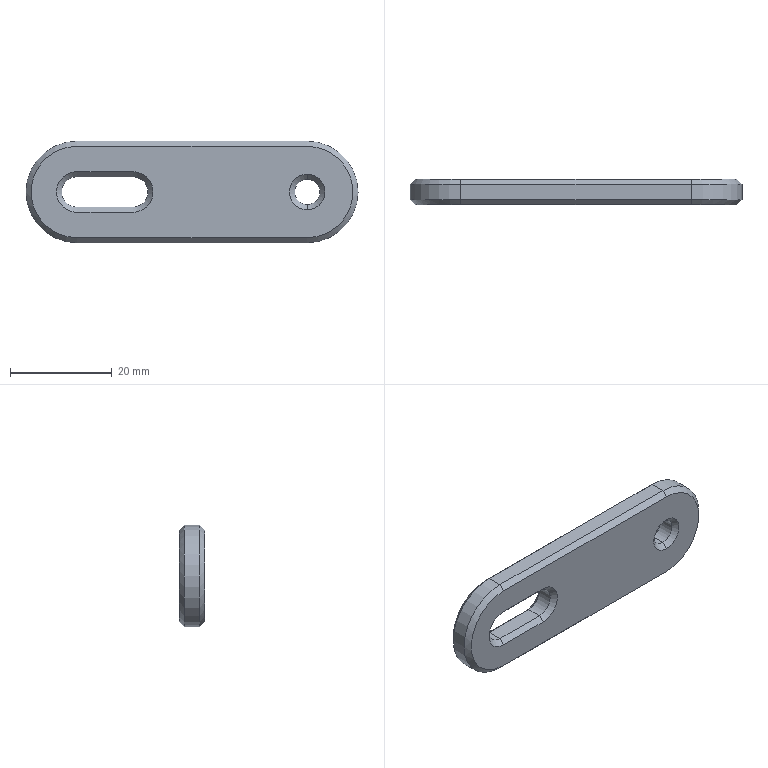Part | SolidWorks | features Chamfer 1, Extrusion 1 | 1 solid | 32 faces | box 65.398 x 5 x 20 mm | volume 5328 mm3 | plane 14 | cone 12 | cylinder 6 | commonest cylinder face diameters 5 x2 6 x2 20 x2
STEP:
#1=CARTESIAN_POINT('',(0.,4.,-2.5));
#2=VERTEX_POINT('',#1);
#3=CARTESIAN_POINT('',(0.,4.,2.5));
#4=VERTEX_POINT('',#3);
#5=CARTESIAN_POINT('',(0.,4.,0.));
#6=DIRECTION('',(0.,1.,0.));
#7=DIRECTION('',(0.,0.,1.));
#8=AXIS2_PLACEMENT_3D('',#5,#6,#7);
#9=CIRCLE('',#8,2.5);
#10=EDGE_CURVE('',#2,#4,#9,.T.);
#11=ORIENTED_EDGE('',*,*,#10,.F.);
#12=CARTESIAN_POINT('',(0.,5.,-3.5));
#13=VERTEX_POINT('',#12);
#14=CARTESIAN_POINT('',(0.,4.,-2.5));
#15=DIRECTION('',(0.,0.7071,-0.7071));
#16=VECTOR('',#15,1000.);
#17=LINE('',#14,#16);
#18=EDGE_CURVE('',#2,#13,#17,.T.);
#19=ORIENTED_EDGE('',*,*,#18,.T.);
#20=CARTESIAN_POINT('',(0.,5.,3.5));
#21=VERTEX_POINT('',#20);
#22=CARTESIAN_POINT('',(0.,5.,0.));
#23=DIRECTION('',(0.,-1.,0.));
#24=DIRECTION('',(0.,0.,1.));
#25=AXIS2_PLACEMENT_3D('',#22,#23,#24);
#26=CIRCLE('',#25,3.5);
#27=EDGE_CURVE('',#21,#13,#26,.T.);
#28=ORIENTED_EDGE('',*,*,#27,.F.);
#29=CARTESIAN_POINT('',(0.,4.,2.5));
#30=DIRECTION('',(0.,0.7071,0.7071));
#31=VECTOR('',#30,1000.);
#32=LINE('',#29,#31);
#33=EDGE_CURVE('',#4,#21,#32,.T.);
#34=ORIENTED_EDGE('',*,*,#33,.F.);
#35=EDGE_LOOP('',(#11,#19,#28,#34));
#36=FACE_OUTER_BOUND('',#35,.T.);
#37=CARTESIAN_POINT('',(0.,4.,0.));
#38=DIRECTION('',(0.,1.,0.));
#39=DIRECTION('',(0.,0.,1.));
#40=AXIS2_PLACEMENT_3D('',#37,#38,#39);
#41=CONICAL_SURFACE('',#40,2.5,0.7854);
#42=ADVANCED_FACE('',(#36),#41,.F.);
#43=CARTESIAN_POINT('',(0.,1.,2.5));
#44=VERTEX_POINT('',#43);
#45=CARTESIAN_POINT('',(0.,1.,-2.5));
#46=VERTEX_POINT('',#45);
#47=CARTESIAN_POINT('',(0.,1.,0.));
#48=DIRECTION('',(0.,-1.,0.));
#49=DIRECTION('',(0.,0.,1.));
#50=AXIS2_PLACEMENT_3D('',#47,#48,#49);
#51=CIRCLE('',#50,2.5);
#52=EDGE_CURVE('',#44,#46,#51,.T.);
#53=ORIENTED_EDGE('',*,*,#52,.F.);
#54=CARTESIAN_POINT('',(0.,0.,3.5));
#55=VERTEX_POINT('',#54);
#56=CARTESIAN_POINT('',(0.,0.,3.5));
#57=DIRECTION('',(0.,-0.7071,0.7071));
#58=VECTOR('',#57,1000.);
#59=LINE('',#56,#58);
#60=EDGE_CURVE('',#44,#55,#59,.T.);
#61=ORIENTED_EDGE('',*,*,#60,.T.);
#62=CARTESIAN_POINT('',(0.,0.,-3.5));
#63=VERTEX_POINT('',#62);
#64=CARTESIAN_POINT('',(0.,0.,0.));
#65=DIRECTION('',(0.,1.,0.));
#66=DIRECTION('',(0.,0.,1.));
#67=AXIS2_PLACEMENT_3D('',#64,#65,#66);
#68=CIRCLE('',#67,3.5);
#69=EDGE_CURVE('',#63,#55,#68,.T.);
#70=ORIENTED_EDGE('',*,*,#69,.F.);
#71=CARTESIAN_POINT('',(0.,0.,-3.5));
#72=DIRECTION('',(0.,-0.7071,-0.7071));
#73=VECTOR('',#72,1000.);
#74=LINE('',#71,#73);
#75=EDGE_CURVE('',#46,#63,#74,.T.);
#76=ORIENTED_EDGE('',*,*,#75,.F.);
#77=EDGE_LOOP('',(#53,#61,#70,#76));
#78=FACE_OUTER_BOUND('',#77,.T.);
#79=CARTESIAN_POINT('',(0.,0.,0.));
#80=DIRECTION('',(0.,-1.,0.));
#81=DIRECTION('',(0.,0.,-1.));
#82=AXIS2_PLACEMENT_3D('',#79,#80,#81);
#83=CONICAL_SURFACE('',#82,3.5,0.7854);
#84=ADVANCED_FACE('',(#78),#83,.F.);
#85=ORIENTED_EDGE('',*,*,#10,.T.);
#86=CARTESIAN_POINT('',(0.,5.,2.5));
#87=DIRECTION('',(0.,-1.,0.));
#88=VECTOR('',#87,1000.);
#89=LINE('',#86,#88);
#90=EDGE_CURVE('',#4,#44,#89,.T.);
#91=ORIENTED_EDGE('',*,*,#90,.T.);
#92=ORIENTED_EDGE('',*,*,#52,.T.);
#93=CARTESIAN_POINT('',(0.,5.,-2.5));
#94=DIRECTION('',(0.,-1.,0.));
#95=VECTOR('',#94,1000.);
#96=LINE('',#93,#95);
#97=EDGE_CURVE('',#2,#46,#96,.T.);
#98=ORIENTED_EDGE('',*,*,#97,.F.);
#99=EDGE_LOOP('',(#85,#91,#92,#98));
#100=FACE_OUTER_BOUND('',#99,.T.);
#101=CARTESIAN_POINT('',(0.,5.,0.));
#102=DIRECTION('',(0.,-1.,0.));
#103=DIRECTION('',(0.,0.,-1.));
#104=AXIS2_PLACEMENT_3D('',#101,#102,#103);
#105=CYLINDRICAL_SURFACE('',#104,2.5);
#106=ADVANCED_FACE('',(#100),#105,.F.);
#107=CARTESIAN_POINT('',(-45.398,5.,-4.));
#108=VERTEX_POINT('',#107);
#109=CARTESIAN_POINT('',(-34.373,5.,-4.));
#110=VERTEX_POINT('',#109);
#111=CARTESIAN_POINT('',(0.,5.,-4.));
#112=DIRECTION('',(1.,0.,0.));
#113=VECTOR('',#112,1000.);
#114=LINE('',#111,#113);
#115=EDGE_CURVE('',#108,#110,#114,.T.);
#116=ORIENTED_EDGE('',*,*,#115,.T.);
#117=CARTESIAN_POINT('',(-34.373,5.,4.));
#118=VERTEX_POINT('',#117);
#119=CARTESIAN_POINT('',(-34.373,5.,0.));
#120=DIRECTION('',(0.,-1.,0.));
#121=DIRECTION('',(0.,0.,1.));
#122=AXIS2_PLACEMENT_3D('',#119,#120,#121);
#123=CIRCLE('',#122,4.);
#124=EDGE_CURVE('',#110,#118,#123,.T.);
#125=ORIENTED_EDGE('',*,*,#124,.T.);
#126=CARTESIAN_POINT('',(-45.398,5.,4.));
#127=VERTEX_POINT('',#126);
#128=CARTESIAN_POINT('',(0.,5.,4.));
#129=DIRECTION('',(-1.,0.,0.));
#130=VECTOR('',#129,1000.);
#131=LINE('',#128,#130);
#132=EDGE_CURVE('',#118,#127,#131,.T.);
#133=ORIENTED_EDGE('',*,*,#132,.T.);
#134=CARTESIAN_POINT('',(-45.398,5.,0.));
#135=DIRECTION('',(0.,-1.,0.));
#136=DIRECTION('',(0.,0.,1.));
#137=AXIS2_PLACEMENT_3D('',#134,#135,#136);
#138=CIRCLE('',#137,4.);
#139=EDGE_CURVE('',#127,#108,#138,.T.);
#140=ORIENTED_EDGE('',*,*,#139,.T.);
#141=EDGE_LOOP('',(#116,#125,#133,#140));
#142=FACE_BOUND('',#141,.T.);
#143=ORIENTED_EDGE('',*,*,#27,.T.);
#144=CARTESIAN_POINT('',(0.,5.,0.));
#145=DIRECTION('',(0.,-1.,0.));
#146=DIRECTION('',(0.,0.,1.));
#147=AXIS2_PLACEMENT_3D('',#144,#145,#146);
#148=CIRCLE('',#147,3.5);
#149=EDGE_CURVE('',#13,#21,#148,.T.);
#150=ORIENTED_EDGE('',*,*,#149,.T.);
#151=EDGE_LOOP('',(#143,#150));
#152=FACE_BOUND('',#151,.T.);
#153=CARTESIAN_POINT('',(-45.398,5.,-9.));
#154=VERTEX_POINT('',#153);
#155=CARTESIAN_POINT('',(-45.398,5.,9.));
#156=VERTEX_POINT('',#155);
#157=CARTESIAN_POINT('',(-45.398,5.,0.));
#158=DIRECTION('',(0.,1.,0.));
#159=DIRECTION('',(0.,0.,1.));
#160=AXIS2_PLACEMENT_3D('',#157,#158,#159);
#161=CIRCLE('',#160,9.);
#162=EDGE_CURVE('',#154,#156,#161,.T.);
#163=ORIENTED_EDGE('',*,*,#162,.T.);
#164=CARTESIAN_POINT('',(0.,5.,9.));
#165=VERTEX_POINT('',#164);
#166=CARTESIAN_POINT('',(0.,5.,9.));
#167=DIRECTION('',(1.,0.,0.));
#168=VECTOR('',#167,1000.);
#169=LINE('',#166,#168);
#170=EDGE_CURVE('',#156,#165,#169,.T.);
#171=ORIENTED_EDGE('',*,*,#170,.T.);
#172=CARTESIAN_POINT('',(0.,5.,-9.));
#173=VERTEX_POINT('',#172);
#174=CARTESIAN_POINT('',(0.,5.,0.));
#175=DIRECTION('',(0.,1.,0.));
#176=DIRECTION('',(0.,0.,1.));
#177=AXIS2_PLACEMENT_3D('',#174,#175,#176);
#178=CIRCLE('',#177,9.);
#179=EDGE_CURVE('',#165,#173,#178,.T.);
#180=ORIENTED_EDGE('',*,*,#179,.T.);
#181=CARTESIAN_POINT('',(-45.398,5.,-9.));
#182=DIRECTION('',(-1.,0.,0.));
#183=VECTOR('',#182,1000.);
#184=LINE('',#181,#183);
#185=EDGE_CURVE('',#173,#154,#184,.T.);
#186=ORIENTED_EDGE('',*,*,#185,.T.);
#187=EDGE_LOOP('',(#163,#171,#180,#186));
#188=FACE_OUTER_BOUND('',#187,.T.);
#189=CARTESIAN_POINT('',(0.,5.,0.));
#190=DIRECTION('',(0.,1.,0.));
#191=DIRECTION('',(0.,0.,1.));
#192=AXIS2_PLACEMENT_3D('',#189,#190,#191);
#193=PLANE('',#192);
#194=ADVANCED_FACE('',(#142,#152,#188),#193,.T.);
#195=CARTESIAN_POINT('',(-34.373,0.,4.));
#196=VERTEX_POINT('',#195);
#197=CARTESIAN_POINT('',(-34.373,0.,-4.));
#198=VERTEX_POINT('',#197);
#199=CARTESIAN_POINT('',(-34.373,0.,0.));
#200=DIRECTION('',(0.,1.,0.));
#201=DIRECTION('',(0.,0.,1.));
#202=AXIS2_PLACEMENT_3D('',#199,#200,#201);
#203=CIRCLE('',#202,4.);
#204=EDGE_CURVE('',#196,#198,#203,.T.);
#205=ORIENTED_EDGE('',*,*,#204,.T.);
#206=CARTESIAN_POINT('',(-45.398,0.,-4.));
#207=VERTEX_POINT('',#206);
#208=CARTESIAN_POINT('',(-45.398,0.,-4.));
#209=DIRECTION('',(-1.,0.,0.));
#210=VECTOR('',#209,1000.);
#211=LINE('',#208,#210);
#212=EDGE_CURVE('',#198,#207,#211,.T.);
#213=ORIENTED_EDGE('',*,*,#212,.T.);
#214=CARTESIAN_POINT('',(-45.398,0.,4.));
#215=VERTEX_POINT('',#214);
#216=CARTESIAN_POINT('',(-45.398,0.,0.));
#217=DIRECTION('',(0.,1.,0.));
#218=DIRECTION('',(0.,0.,1.));
#219=AXIS2_PLACEMENT_3D('',#216,#217,#218);
#220=CIRCLE('',#219,4.);
#221=EDGE_CURVE('',#207,#215,#220,.T.);
#222=ORIENTED_EDGE('',*,*,#221,.T.);
#223=CARTESIAN_POINT('',(-34.373,0.,4.));
#224=DIRECTION('',(1.,0.,0.));
#225=VECTOR('',#224,1000.);
#226=LINE('',#223,#225);
#227=EDGE_CURVE('',#215,#196,#226,.T.);
#228=ORIENTED_EDGE('',*,*,#227,.T.);
#229=EDGE_LOOP('',(#205,#213,#222,#228));
#230=FACE_BOUND('',#229,.T.);
#231=CARTESIAN_POINT('',(-45.398,0.,9.));
#232=VERTEX_POINT('',#231);
#233=CARTESIAN_POINT('',(-45.398,0.,-9.));
#234=VERTEX_POINT('',#233);
#235=CARTESIAN_POINT('',(-45.398,0.,0.));
#236=DIRECTION('',(0.,-1.,0.));
#237=DIRECTION('',(0.,0.,1.));
#238=AXIS2_PLACEMENT_3D('',#235,#236,#237);
#239=CIRCLE('',#238,9.);
#240=EDGE_CURVE('',#232,#234,#239,.T.);
#241=ORIENTED_EDGE('',*,*,#240,.T.);
#242=CARTESIAN_POINT('',(0.,0.,-9.));
#243=VERTEX_POINT('',#242);
#244=CARTESIAN_POINT('',(0.,0.,-9.));
#245=DIRECTION('',(1.,0.,0.));
#246=VECTOR('',#245,1000.);
#247=LINE('',#244,#246);
#248=EDGE_CURVE('',#234,#243,#247,.T.);
#249=ORIENTED_EDGE('',*,*,#248,.T.);
#250=CARTESIAN_POINT('',(0.,0.,9.));
#251=VERTEX_POINT('',#250);
#252=CARTESIAN_POINT('',(0.,0.,0.));
#253=DIRECTION('',(0.,-1.,0.));
#254=DIRECTION('',(0.,0.,1.));
#255=AXIS2_PLACEMENT_3D('',#252,#253,#254);
#256=CIRCLE('',#255,9.);
#257=EDGE_CURVE('',#243,#251,#256,.T.);
#258=ORIENTED_EDGE('',*,*,#257,.T.);
#259=CARTESIAN_POINT('',(0.,0.,9.));
#260=DIRECTION('',(-1.,0.,0.));
#261=VECTOR('',#260,1000.);
#262=LINE('',#259,#261);
#263=EDGE_CURVE('',#251,#232,#262,.T.);
#264=ORIENTED_EDGE('',*,*,#263,.T.);
#265=EDGE_LOOP('',(#241,#249,#258,#264));
#266=FACE_OUTER_BOUND('',#265,.T.);
#267=ORIENTED_EDGE('',*,*,#69,.T.);
#268=CARTESIAN_POINT('',(0.,0.,0.));
#269=DIRECTION('',(0.,1.,0.));
#270=DIRECTION('',(0.,0.,1.));
#271=AXIS2_PLACEMENT_3D('',#268,#269,#270);
#272=CIRCLE('',#271,3.5);
#273=EDGE_CURVE('',#55,#63,#272,.T.);
#274=ORIENTED_EDGE('',*,*,#273,.T.);
#275=EDGE_LOOP('',(#267,#274));
#276=FACE_BOUND('',#275,.T.);
#277=CARTESIAN_POINT('',(0.,0.,0.));
#278=DIRECTION('',(0.,1.,0.));
#279=DIRECTION('',(0.,0.,1.));
#280=AXIS2_PLACEMENT_3D('',#277,#278,#279);
#281=PLANE('',#280);
#282=ADVANCED_FACE('',(#230,#266,#276),#281,.F.);
#283=CARTESIAN_POINT('',(0.,4.,10.));
#284=VERTEX_POINT('',#283);
#285=CARTESIAN_POINT('',(0.,1.,10.));
#286=VERTEX_POINT('',#285);
#287=CARTESIAN_POINT('',(0.,5.,10.));
#288=DIRECTION('',(0.,-1.,0.));
#289=VECTOR('',#288,1000.);
#290=LINE('',#287,#289);
#291=EDGE_CURVE('',#284,#286,#290,.T.);
#292=ORIENTED_EDGE('',*,*,#291,.T.);
#293=CARTESIAN_POINT('',(0.,1.,-10.));
#294=VERTEX_POINT('',#293);
#295=CARTESIAN_POINT('',(0.,1.,0.));
#296=DIRECTION('',(0.,1.,0.));
#297=DIRECTION('',(0.,0.,1.));
#298=AXIS2_PLACEMENT_3D('',#295,#296,#297);
#299=CIRCLE('',#298,10.);
#300=EDGE_CURVE('',#286,#294,#299,.T.);
#301=ORIENTED_EDGE('',*,*,#300,.T.);
#302=CARTESIAN_POINT('',(0.,4.,-10.));
#303=VERTEX_POINT('',#302);
#304=CARTESIAN_POINT('',(0.,5.,-10.));
#305=DIRECTION('',(0.,-1.,0.));
#306=VECTOR('',#305,1000.);
#307=LINE('',#304,#306);
#308=EDGE_CURVE('',#303,#294,#307,.T.);
#309=ORIENTED_EDGE('',*,*,#308,.F.);
#310=CARTESIAN_POINT('',(0.,4.,0.));
#311=DIRECTION('',(0.,-1.,0.));
#312=DIRECTION('',(0.,0.,1.));
#313=AXIS2_PLACEMENT_3D('',#310,#311,#312);
#314=CIRCLE('',#313,10.);
#315=EDGE_CURVE('',#303,#284,#314,.T.);
#316=ORIENTED_EDGE('',*,*,#315,.T.);
#317=EDGE_LOOP('',(#292,#301,#309,#316));
#318=FACE_OUTER_BOUND('',#317,.T.);
#319=CARTESIAN_POINT('',(0.,5.,0.));
#320=DIRECTION('',(0.,-1.,0.));
#321=DIRECTION('',(0.,0.,-1.));
#322=AXIS2_PLACEMENT_3D('',#319,#320,#321);
#323=CYLINDRICAL_SURFACE('',#322,10.);
#324=ADVANCED_FACE('',(#318),#323,.T.);
#325=ORIENTED_EDGE('',*,*,#308,.T.);
#326=CARTESIAN_POINT('',(-45.398,1.,-10.));
#327=VERTEX_POINT('',#326);
#328=CARTESIAN_POINT('',(0.,1.,-10.));
#329=DIRECTION('',(-1.,0.,0.));
#330=VECTOR('',#329,1000.);
#331=LINE('',#328,#330);
#332=EDGE_CURVE('',#294,#327,#331,.T.);
#333=ORIENTED_EDGE('',*,*,#332,.T.);
#334=CARTESIAN_POINT('',(-45.398,4.,-10.));
#335=VERTEX_POINT('',#334);
#336=CARTESIAN_POINT('',(-45.398,5.,-10.));
#337=DIRECTION('',(0.,-1.,0.));
#338=VECTOR('',#337,1000.);
#339=LINE('',#336,#338);
#340=EDGE_CURVE('',#335,#327,#339,.T.);
#341=ORIENTED_EDGE('',*,*,#340,.F.);
#342=CARTESIAN_POINT('',(0.,4.,-10.));
#343=DIRECTION('',(1.,0.,0.));
#344=VECTOR('',#343,1000.);
#345=LINE('',#342,#344);
#346=EDGE_CURVE('',#335,#303,#345,.T.);
#347=ORIENTED_EDGE('',*,*,#346,.T.);
#348=EDGE_LOOP('',(#325,#333,#341,#347));
#349=FACE_OUTER_BOUND('',#348,.T.);
#350=CARTESIAN_POINT('',(0.,5.,-10.));
#351=DIRECTION('',(0.,0.,1.));
#352=DIRECTION('',(1.,0.,0.));
#353=AXIS2_PLACEMENT_3D('',#350,#351,#352);
#354=PLANE('',#353);
#355=ADVANCED_FACE('',(#349),#354,.F.);
#356=ORIENTED_EDGE('',*,*,#340,.T.);
#357=CARTESIAN_POINT('',(-45.398,1.,10.));
#358=VERTEX_POINT('',#357);
#359=CARTESIAN_POINT('',(-45.398,1.,0.));
#360=DIRECTION('',(0.,1.,0.));
#361=DIRECTION('',(0.,0.,1.));
#362=AXIS2_PLACEMENT_3D('',#359,#360,#361);
#363=CIRCLE('',#362,10.);
#364=EDGE_CURVE('',#327,#358,#363,.T.);
#365=ORIENTED_EDGE('',*,*,#364,.T.);
#366=CARTESIAN_POINT('',(-45.398,4.,10.));
#367=VERTEX_POINT('',#366);
#368=CARTESIAN_POINT('',(-45.398,5.,10.));
#369=DIRECTION('',(0.,-1.,0.));
#370=VECTOR('',#369,1000.);
#371=LINE('',#368,#370);
#372=EDGE_CURVE('',#367,#358,#371,.T.);
#373=ORIENTED_EDGE('',*,*,#372,.F.);
#374=CARTESIAN_POINT('',(-45.398,4.,0.));
#375=DIRECTION('',(0.,-1.,0.));
#376=DIRECTION('',(0.,0.,1.));
#377=AXIS2_PLACEMENT_3D('',#374,#375,#376);
#378=CIRCLE('',#377,10.);
#379=EDGE_CURVE('',#367,#335,#378,.T.);
#380=ORIENTED_EDGE('',*,*,#379,.T.);
#381=EDGE_LOOP('',(#356,#365,#373,#380));
#382=FACE_OUTER_BOUND('',#381,.T.);
#383=CARTESIAN_POINT('',(-45.398,5.,0.));
#384=DIRECTION('',(0.,-1.,0.));
#385=DIRECTION('',(0.,0.,-1.));
#386=AXIS2_PLACEMENT_3D('',#383,#384,#385);
#387=CYLINDRICAL_SURFACE('',#386,10.);
#388=ADVANCED_FACE('',(#382),#387,.T.);
#389=ORIENTED_EDGE('',*,*,#372,.T.);
#390=CARTESIAN_POINT('',(0.,1.,10.));
#391=DIRECTION('',(1.,0.,0.));
#392=VECTOR('',#391,1000.);
#393=LINE('',#390,#392);
#394=EDGE_CURVE('',#358,#286,#393,.T.);
#395=ORIENTED_EDGE('',*,*,#394,.T.);
#396=ORIENTED_EDGE('',*,*,#291,.F.);
#397=CARTESIAN_POINT('',(-45.398,4.,10.));
#398=DIRECTION('',(-1.,0.,0.));
#399=VECTOR('',#398,1000.);
#400=LINE('',#397,#399);
#401=EDGE_CURVE('',#284,#367,#400,.T.);
#402=ORIENTED_EDGE('',*,*,#401,.T.);
#403=EDGE_LOOP('',(#389,#395,#396,#402));
#404=FACE_OUTER_BOUND('',#403,.T.);
#405=CARTESIAN_POINT('',(0.,5.,10.));
#406=DIRECTION('',(0.,0.,-1.));
#407=DIRECTION('',(-1.,0.,0.));
#408=AXIS2_PLACEMENT_3D('',#405,#406,#407);
#409=PLANE('',#408);
#410=ADVANCED_FACE('',(#404),#409,.F.);
#411=ORIENTED_EDGE('',*,*,#90,.F.);
#412=CARTESIAN_POINT('',(0.,4.,0.));
#413=DIRECTION('',(0.,1.,0.));
#414=DIRECTION('',(0.,0.,1.));
#415=AXIS2_PLACEMENT_3D('',#412,#413,#414);
#416=CIRCLE('',#415,2.5);
#417=EDGE_CURVE('',#4,#2,#416,.T.);
#418=ORIENTED_EDGE('',*,*,#417,.T.);
#419=ORIENTED_EDGE('',*,*,#97,.T.);
#420=CARTESIAN_POINT('',(0.,1.,0.));
#421=DIRECTION('',(0.,-1.,0.));
#422=DIRECTION('',(0.,0.,1.));
#423=AXIS2_PLACEMENT_3D('',#420,#421,#422);
#424=CIRCLE('',#423,2.5);
#425=EDGE_CURVE('',#46,#44,#424,.T.);
#426=ORIENTED_EDGE('',*,*,#425,.T.);
#427=EDGE_LOOP('',(#411,#418,#419,#426));
#428=FACE_OUTER_BOUND('',#427,.T.);
#429=CARTESIAN_POINT('',(0.,5.,0.));
#430=DIRECTION('',(0.,-1.,0.));
#431=DIRECTION('',(0.,0.,-1.));
#432=AXIS2_PLACEMENT_3D('',#429,#430,#431);
#433=CYLINDRICAL_SURFACE('',#432,2.5);
#434=ADVANCED_FACE('',(#428),#433,.F.);
#435=CARTESIAN_POINT('',(-45.398,4.,3.));
#436=VERTEX_POINT('',#435);
#437=CARTESIAN_POINT('',(-45.398,1.,3.));
#438=VERTEX_POINT('',#437);
#439=CARTESIAN_POINT('',(-45.398,5.,3.));
#440=DIRECTION('',(0.,-1.,0.));
#441=VECTOR('',#440,1000.);
#442=LINE('',#439,#441);
#443=EDGE_CURVE('',#436,#438,#442,.T.);
#444=ORIENTED_EDGE('',*,*,#443,.T.);
#445=CARTESIAN_POINT('',(-45.398,1.,-3.));
#446=VERTEX_POINT('',#445);
#447=CARTESIAN_POINT('',(-45.398,1.,0.));
#448=DIRECTION('',(0.,-1.,0.));
#449=DIRECTION('',(0.,0.,1.));
#450=AXIS2_PLACEMENT_3D('',#447,#448,#449);
#451=CIRCLE('',#450,3.);
#452=EDGE_CURVE('',#438,#446,#451,.T.);
#453=ORIENTED_EDGE('',*,*,#452,.T.);
#454=CARTESIAN_POINT('',(-45.398,4.,-3.));
#455=VERTEX_POINT('',#454);
#456=CARTESIAN_POINT('',(-45.398,5.,-3.));
#457=DIRECTION('',(0.,-1.,0.));
#458=VECTOR('',#457,1000.);
#459=LINE('',#456,#458);
#460=EDGE_CURVE('',#455,#446,#459,.T.);
#461=ORIENTED_EDGE('',*,*,#460,.F.);
#462=CARTESIAN_POINT('',(-45.398,4.,0.));
#463=DIRECTION('',(0.,1.,0.));
#464=DIRECTION('',(0.,0.,1.));
#465=AXIS2_PLACEMENT_3D('',#462,#463,#464);
#466=CIRCLE('',#465,3.);
#467=EDGE_CURVE('',#455,#436,#466,.T.);
#468=ORIENTED_EDGE('',*,*,#467,.T.);
#469=EDGE_LOOP('',(#444,#453,#461,#468));
#470=FACE_OUTER_BOUND('',#469,.T.);
#471=CARTESIAN_POINT('',(-45.398,5.,0.));
#472=DIRECTION('',(0.,-1.,0.));
#473=DIRECTION('',(0.,0.,-1.));
#474=AXIS2_PLACEMENT_3D('',#471,#472,#473);
#475=CYLINDRICAL_SURFACE('',#474,3.);
#476=ADVANCED_FACE('',(#470),#475,.F.);
#477=CARTESIAN_POINT('',(-34.373,4.,3.));
#478=VERTEX_POINT('',#477);
#479=CARTESIAN_POINT('',(-34.373,1.,3.));
#480=VERTEX_POINT('',#479);
#481=CARTESIAN_POINT('',(-34.373,5.,3.));
#482=DIRECTION('',(0.,-1.,0.));
#483=VECTOR('',#482,1000.);
#484=LINE('',#481,#483);
#485=EDGE_CURVE('',#478,#480,#484,.T.);
#486=ORIENTED_EDGE('',*,*,#485,.T.);
#487=CARTESIAN_POINT('',(-45.398,1.,3.));
#488=DIRECTION('',(-1.,0.,0.));
#489=VECTOR('',#488,1000.);
#490=LINE('',#487,#489);
#491=EDGE_CURVE('',#480,#438,#490,.T.);
#492=ORIENTED_EDGE('',*,*,#491,.T.);
#493=ORIENTED_EDGE('',*,*,#443,.F.);
#494=CARTESIAN_POINT('',(-45.398,4.,3.));
#495=DIRECTION('',(1.,0.,0.));
#496=VECTOR('',#495,1000.);
#497=LINE('',#494,#496);
#498=EDGE_CURVE('',#436,#478,#497,.T.);
#499=ORIENTED_EDGE('',*,*,#498,.T.);
#500=EDGE_LOOP('',(#486,#492,#493,#499));
#501=FACE_OUTER_BOUND('',#500,.T.);
#502=CARTESIAN_POINT('',(-45.398,5.,3.));
#503=DIRECTION('',(0.,0.,-1.));
#504=DIRECTION('',(-1.,0.,0.));
#505=AXIS2_PLACEMENT_3D('',#502,#503,#504);
#506=PLANE('',#505);
#507=ADVANCED_FACE('',(#501),#506,.T.);
#508=CARTESIAN_POINT('',(-34.373,4.,-3.));
#509=VERTEX_POINT('',#508);
#510=CARTESIAN_POINT('',(-34.373,1.,-3.));
#511=VERTEX_POINT('',#510);
#512=CARTESIAN_POINT('',(-34.373,5.,-3.));
#513=DIRECTION('',(0.,-1.,0.));
#514=VECTOR('',#513,1000.);
#515=LINE('',#512,#514);
#516=EDGE_CURVE('',#509,#511,#515,.T.);
#517=ORIENTED_EDGE('',*,*,#516,.T.);
#518=CARTESIAN_POINT('',(-34.373,1.,0.));
#519=DIRECTION('',(0.,-1.,0.));
#520=DIRECTION('',(0.,0.,1.));
#521=AXIS2_PLACEMENT_3D('',#518,#519,#520);
#522=CIRCLE('',#521,3.);
#523=EDGE_CURVE('',#511,#480,#522,.T.);
#524=ORIENTED_EDGE('',*,*,#523,.T.);
#525=ORIENTED_EDGE('',*,*,#485,.F.);
#526=CARTESIAN_POINT('',(-34.373,4.,0.));
#527=DIRECTION('',(0.,1.,0.));
#528=DIRECTION('',(0.,0.,1.));
#529=AXIS2_PLACEMENT_3D('',#526,#527,#528);
#530=CIRCLE('',#529,3.);
#531=EDGE_CURVE('',#478,#509,#530,.T.);
#532=ORIENTED_EDGE('',*,*,#531,.T.);
#533=EDGE_LOOP('',(#517,#524,#525,#532));
#534=FACE_OUTER_BOUND('',#533,.T.);
#535=CARTESIAN_POINT('',(-34.373,5.,0.));
#536=DIRECTION('',(0.,-1.,0.));
#537=DIRECTION('',(0.,0.,-1.));
#538=AXIS2_PLACEMENT_3D('',#535,#536,#537);
#539=CYLINDRICAL_SURFACE('',#538,3.);
#540=ADVANCED_FACE('',(#534),#539,.F.);
#541=ORIENTED_EDGE('',*,*,#460,.T.);
#542=CARTESIAN_POINT('',(-34.373,1.,-3.));
#543=DIRECTION('',(1.,0.,0.));
#544=VECTOR('',#543,1000.);
#545=LINE('',#542,#544);
#546=EDGE_CURVE('',#446,#511,#545,.T.);
#547=ORIENTED_EDGE('',*,*,#546,.T.);
#548=ORIENTED_EDGE('',*,*,#516,.F.);
#549=CARTESIAN_POINT('',(-45.398,4.,-3.));
#550=DIRECTION('',(-1.,0.,0.));
#551=VECTOR('',#550,1000.);
#552=LINE('',#549,#551);
#553=EDGE_CURVE('',#509,#455,#552,.T.);
#554=ORIENTED_EDGE('',*,*,#553,.T.);
#555=EDGE_LOOP('',(#541,#547,#548,#554));
#556=FACE_OUTER_BOUND('',#555,.T.);
#557=CARTESIAN_POINT('',(-45.398,5.,-3.));
#558=DIRECTION('',(0.,0.,1.));
#559=DIRECTION('',(1.,0.,0.));
#560=AXIS2_PLACEMENT_3D('',#557,#558,#559);
#561=PLANE('',#560);
#562=ADVANCED_FACE('',(#556),#561,.T.);
#563=CARTESIAN_POINT('',(-45.398,1.,3.));
#564=DIRECTION('',(0.,-0.7071,0.7071));
#565=VECTOR('',#564,1000.);
#566=LINE('',#563,#565);
#567=EDGE_CURVE('',#438,#215,#566,.T.);
#568=ORIENTED_EDGE('',*,*,#567,.F.);
#569=ORIENTED_EDGE('',*,*,#491,.F.);
#570=CARTESIAN_POINT('',(-34.373,0.,4.));
#571=DIRECTION('',(0.,0.7071,-0.7071));
#572=VECTOR('',#571,1000.);
#573=LINE('',#570,#572);
#574=EDGE_CURVE('',#196,#480,#573,.T.);
#575=ORIENTED_EDGE('',*,*,#574,.F.);
#576=ORIENTED_EDGE('',*,*,#227,.F.);
#577=EDGE_LOOP('',(#568,#569,#575,#576));
#578=FACE_OUTER_BOUND('',#577,.T.);
#579=CARTESIAN_POINT('',(0.,0.,4.));
#580=DIRECTION('',(0.,-0.7071,-0.7071));
#581=DIRECTION('',(-1.,0.,0.));
#582=AXIS2_PLACEMENT_3D('',#579,#580,#581);
#583=PLANE('',#582);
#584=ADVANCED_FACE('',(#578),#583,.T.);
#585=ORIENTED_EDGE('',*,*,#574,.T.);
#586=ORIENTED_EDGE('',*,*,#523,.F.);
#587=CARTESIAN_POINT('',(-34.373,0.,-4.));
#588=DIRECTION('',(0.,0.7071,0.7071));
#589=VECTOR('',#588,1000.);
#590=LINE('',#587,#589);
#591=EDGE_CURVE('',#198,#511,#590,.T.);
#592=ORIENTED_EDGE('',*,*,#591,.F.);
#593=ORIENTED_EDGE('',*,*,#204,.F.);
#594=EDGE_LOOP('',(#585,#586,#592,#593));
#595=FACE_OUTER_BOUND('',#594,.T.);
#596=CARTESIAN_POINT('',(-34.373,0.,0.));
#597=DIRECTION('',(0.,-1.,0.));
#598=DIRECTION('',(0.,0.,-1.));
#599=AXIS2_PLACEMENT_3D('',#596,#597,#598);
#600=CONICAL_SURFACE('',#599,4.,0.7854);
#601=ADVANCED_FACE('',(#595),#600,.F.);
#602=ORIENTED_EDGE('',*,*,#567,.T.);
#603=ORIENTED_EDGE('',*,*,#221,.F.);
#604=CARTESIAN_POINT('',(-45.398,1.,-3.));
#605=DIRECTION('',(0.,-0.7071,-0.7071));
#606=VECTOR('',#605,1000.);
#607=LINE('',#604,#606);
#608=EDGE_CURVE('',#446,#207,#607,.T.);
#609=ORIENTED_EDGE('',*,*,#608,.F.);
#610=ORIENTED_EDGE('',*,*,#452,.F.);
#611=EDGE_LOOP('',(#602,#603,#609,#610));
#612=FACE_OUTER_BOUND('',#611,.T.);
#613=CARTESIAN_POINT('',(-45.398,0.,0.));
#614=DIRECTION('',(0.,-1.,0.));
#615=DIRECTION('',(0.,0.,-1.));
#616=AXIS2_PLACEMENT_3D('',#613,#614,#615);
#617=CONICAL_SURFACE('',#616,4.,0.7854);
#618=ADVANCED_FACE('',(#612),#617,.F.);
#619=ORIENTED_EDGE('',*,*,#591,.T.);
#620=ORIENTED_EDGE('',*,*,#546,.F.);
#621=ORIENTED_EDGE('',*,*,#608,.T.);
#622=ORIENTED_EDGE('',*,*,#212,.F.);
#623=EDGE_LOOP('',(#619,#620,#621,#622));
#624=FACE_OUTER_BOUND('',#623,.T.);
#625=CARTESIAN_POINT('',(0.,0.,-4.));
#626=DIRECTION('',(0.,-0.7071,0.7071));
#627=DIRECTION('',(1.,0.,0.));
#628=AXIS2_PLACEMENT_3D('',#625,#626,#627);
#629=PLANE('',#628);
#630=ADVANCED_FACE('',(#624),#629,.T.);
#631=CARTESIAN_POINT('',(-45.398,0.,9.));
#632=DIRECTION('',(0.,0.7071,0.7071));
#633=VECTOR('',#632,1000.);
#634=LINE('',#631,#633);
#635=EDGE_CURVE('',#232,#358,#634,.T.);
#636=ORIENTED_EDGE('',*,*,#635,.F.);
#637=ORIENTED_EDGE('',*,*,#263,.F.);
#638=CARTESIAN_POINT('',(0.,1.,10.));
#639=DIRECTION('',(0.,-0.7071,-0.7071));
#640=VECTOR('',#639,1000.);
#641=LINE('',#638,#640);
#642=EDGE_CURVE('',#286,#251,#641,.T.);
#643=ORIENTED_EDGE('',*,*,#642,.F.);
#644=ORIENTED_EDGE('',*,*,#394,.F.);
#645=EDGE_LOOP('',(#636,#637,#643,#644));
#646=FACE_OUTER_BOUND('',#645,.T.);
#647=CARTESIAN_POINT('',(0.,1.,10.));
#648=DIRECTION('',(0.,0.7071,-0.7071));
#649=DIRECTION('',(1.,0.,0.));
#650=AXIS2_PLACEMENT_3D('',#647,#648,#649);
#651=PLANE('',#650);
#652=ADVANCED_FACE('',(#646),#651,.F.);
#653=ORIENTED_EDGE('',*,*,#642,.T.);
#654=ORIENTED_EDGE('',*,*,#257,.F.);
#655=CARTESIAN_POINT('',(0.,1.,-10.));
#656=DIRECTION('',(0.,-0.7071,0.7071));
#657=VECTOR('',#656,1000.);
#658=LINE('',#655,#657);
#659=EDGE_CURVE('',#294,#243,#658,.T.);
#660=ORIENTED_EDGE('',*,*,#659,.F.);
#661=ORIENTED_EDGE('',*,*,#300,.F.);
#662=EDGE_LOOP('',(#653,#654,#660,#661));
#663=FACE_OUTER_BOUND('',#662,.T.);
#664=CARTESIAN_POINT('',(0.,1.,0.));
#665=DIRECTION('',(0.,1.,0.));
#666=DIRECTION('',(0.,0.,1.));
#667=AXIS2_PLACEMENT_3D('',#664,#665,#666);
#668=CONICAL_SURFACE('',#667,10.,0.7854);
#669=ADVANCED_FACE('',(#663),#668,.T.);
#670=ORIENTED_EDGE('',*,*,#635,.T.);
#671=ORIENTED_EDGE('',*,*,#364,.F.);
#672=CARTESIAN_POINT('',(-45.398,0.,-9.));
#673=DIRECTION('',(0.,0.7071,-0.7071));
#674=VECTOR('',#673,1000.);
#675=LINE('',#672,#674);
#676=EDGE_CURVE('',#234,#327,#675,.T.);
#677=ORIENTED_EDGE('',*,*,#676,.F.);
#678=ORIENTED_EDGE('',*,*,#240,.F.);
#679=EDGE_LOOP('',(#670,#671,#677,#678));
#680=FACE_OUTER_BOUND('',#679,.T.);
#681=CARTESIAN_POINT('',(-45.398,1.,0.));
#682=DIRECTION('',(0.,1.,0.));
#683=DIRECTION('',(0.,0.,1.));
#684=AXIS2_PLACEMENT_3D('',#681,#682,#683);
#685=CONICAL_SURFACE('',#684,10.,0.7854);
#686=ADVANCED_FACE('',(#680),#685,.T.);
#687=ORIENTED_EDGE('',*,*,#659,.T.);
#688=ORIENTED_EDGE('',*,*,#248,.F.);
#689=ORIENTED_EDGE('',*,*,#676,.T.);
#690=ORIENTED_EDGE('',*,*,#332,.F.);
#691=EDGE_LOOP('',(#687,#688,#689,#690));
#692=FACE_OUTER_BOUND('',#691,.T.);
#693=CARTESIAN_POINT('',(0.,1.,-10.));
#694=DIRECTION('',(0.,0.7071,0.7071));
#695=DIRECTION('',(-1.,0.,0.));
#696=AXIS2_PLACEMENT_3D('',#693,#694,#695);
#697=PLANE('',#696);
#698=ADVANCED_FACE('',(#692),#697,.F.);
#699=ORIENTED_EDGE('',*,*,#60,.F.);
#700=ORIENTED_EDGE('',*,*,#425,.F.);
#701=ORIENTED_EDGE('',*,*,#75,.T.);
#702=ORIENTED_EDGE('',*,*,#273,.F.);
#703=EDGE_LOOP('',(#699,#700,#701,#702));
#704=FACE_OUTER_BOUND('',#703,.T.);
#705=CARTESIAN_POINT('',(0.,0.,0.));
#706=DIRECTION('',(0.,-1.,0.));
#707=DIRECTION('',(0.,0.,-1.));
#708=AXIS2_PLACEMENT_3D('',#705,#706,#707);
#709=CONICAL_SURFACE('',#708,3.5,0.7854);
#710=ADVANCED_FACE('',(#704),#709,.F.);
#711=CARTESIAN_POINT('',(-45.398,5.,-4.));
#712=DIRECTION('',(0.,-0.7071,0.7071));
#713=VECTOR('',#712,1000.);
#714=LINE('',#711,#713);
#715=EDGE_CURVE('',#108,#455,#714,.T.);
#716=ORIENTED_EDGE('',*,*,#715,.F.);
#717=ORIENTED_EDGE('',*,*,#139,.F.);
#718=CARTESIAN_POINT('',(-45.398,4.,3.));
#719=DIRECTION('',(0.,0.7071,0.7071));
#720=VECTOR('',#719,1000.);
#721=LINE('',#718,#720);
#722=EDGE_CURVE('',#436,#127,#721,.T.);
#723=ORIENTED_EDGE('',*,*,#722,.F.);
#724=ORIENTED_EDGE('',*,*,#467,.F.);
#725=EDGE_LOOP('',(#716,#717,#723,#724));
#726=FACE_OUTER_BOUND('',#725,.T.);
#727=CARTESIAN_POINT('',(-45.398,4.,0.));
#728=DIRECTION('',(0.,1.,0.));
#729=DIRECTION('',(0.,0.,1.));
#730=AXIS2_PLACEMENT_3D('',#727,#728,#729);
#731=CONICAL_SURFACE('',#730,3.,0.7854);
#732=ADVANCED_FACE('',(#726),#731,.F.);
#733=ORIENTED_EDGE('',*,*,#722,.T.);
#734=ORIENTED_EDGE('',*,*,#132,.F.);
#735=CARTESIAN_POINT('',(-34.373,4.,3.));
#736=DIRECTION('',(0.,0.7071,0.7071));
#737=VECTOR('',#736,1000.);
#738=LINE('',#735,#737);
#739=EDGE_CURVE('',#478,#118,#738,.T.);
#740=ORIENTED_EDGE('',*,*,#739,.F.);
#741=ORIENTED_EDGE('',*,*,#498,.F.);
#742=EDGE_LOOP('',(#733,#734,#740,#741));
#743=FACE_OUTER_BOUND('',#742,.T.);
#744=CARTESIAN_POINT('',(-45.398,4.,3.));
#745=DIRECTION('',(0.,-0.7071,0.7071));
#746=DIRECTION('',(1.,0.,0.));
#747=AXIS2_PLACEMENT_3D('',#744,#745,#746);
#748=PLANE('',#747);
#749=ADVANCED_FACE('',(#743),#748,.F.);
#750=ORIENTED_EDGE('',*,*,#715,.T.);
#751=ORIENTED_EDGE('',*,*,#553,.F.);
#752=CARTESIAN_POINT('',(-34.373,5.,-4.));
#753=DIRECTION('',(0.,-0.7071,0.7071));
#754=VECTOR('',#753,1000.);
#755=LINE('',#752,#754);
#756=EDGE_CURVE('',#110,#509,#755,.T.);
#757=ORIENTED_EDGE('',*,*,#756,.F.);
#758=ORIENTED_EDGE('',*,*,#115,.F.);
#759=EDGE_LOOP('',(#750,#751,#757,#758));
#760=FACE_OUTER_BOUND('',#759,.T.);
#761=CARTESIAN_POINT('',(-45.398,4.,-3.));
#762=DIRECTION('',(0.,-0.7071,-0.7071));
#763=DIRECTION('',(-1.,0.,0.));
#764=AXIS2_PLACEMENT_3D('',#761,#762,#763);
#765=PLANE('',#764);
#766=ADVANCED_FACE('',(#760),#765,.F.);
#767=ORIENTED_EDGE('',*,*,#739,.T.);
#768=ORIENTED_EDGE('',*,*,#124,.F.);
#769=ORIENTED_EDGE('',*,*,#756,.T.);
#770=ORIENTED_EDGE('',*,*,#531,.F.);
#771=EDGE_LOOP('',(#767,#768,#769,#770));
#772=FACE_OUTER_BOUND('',#771,.T.);
#773=CARTESIAN_POINT('',(-34.373,4.,0.));
#774=DIRECTION('',(0.,1.,0.));
#775=DIRECTION('',(0.,0.,1.));
#776=AXIS2_PLACEMENT_3D('',#773,#774,#775);
#777=CONICAL_SURFACE('',#776,3.,0.7854);
#778=ADVANCED_FACE('',(#772),#777,.F.);
#779=ORIENTED_EDGE('',*,*,#18,.F.);
#780=ORIENTED_EDGE('',*,*,#417,.F.);
#781=ORIENTED_EDGE('',*,*,#33,.T.);
#782=ORIENTED_EDGE('',*,*,#149,.F.);
#783=EDGE_LOOP('',(#779,#780,#781,#782));
#784=FACE_OUTER_BOUND('',#783,.T.);
#785=CARTESIAN_POINT('',(0.,4.,0.));
#786=DIRECTION('',(0.,1.,0.));
#787=DIRECTION('',(0.,0.,1.));
#788=AXIS2_PLACEMENT_3D('',#785,#786,#787);
#789=CONICAL_SURFACE('',#788,2.5,0.7854);
#790=ADVANCED_FACE('',(#784),#789,.F.);
#791=CARTESIAN_POINT('',(0.,4.,-10.));
#792=DIRECTION('',(0.,0.7071,0.7071));
#793=VECTOR('',#792,1000.);
#794=LINE('',#791,#793);
#795=EDGE_CURVE('',#303,#173,#794,.T.);
#796=ORIENTED_EDGE('',*,*,#795,.F.);
#797=ORIENTED_EDGE('',*,*,#346,.F.);
#798=CARTESIAN_POINT('',(-45.398,5.,-9.));
#799=DIRECTION('',(0.,-0.7071,-0.7071));
#800=VECTOR('',#799,1000.);
#801=LINE('',#798,#800);
#802=EDGE_CURVE('',#154,#335,#801,.T.);
#803=ORIENTED_EDGE('',*,*,#802,.F.);
#804=ORIENTED_EDGE('',*,*,#185,.F.);
#805=EDGE_LOOP('',(#796,#797,#803,#804));
#806=FACE_OUTER_BOUND('',#805,.T.);
#807=CARTESIAN_POINT('',(0.,5.,-9.));
#808=DIRECTION('',(0.,0.7071,-0.7071));
#809=DIRECTION('',(1.,0.,0.));
#810=AXIS2_PLACEMENT_3D('',#807,#808,#809);
#811=PLANE('',#810);
#812=ADVANCED_FACE('',(#806),#811,.T.);
#813=ORIENTED_EDGE('',*,*,#802,.T.);
#814=ORIENTED_EDGE('',*,*,#379,.F.);
#815=CARTESIAN_POINT('',(-45.398,5.,9.));
#816=DIRECTION('',(0.,-0.7071,0.7071));
#817=VECTOR('',#816,1000.);
#818=LINE('',#815,#817);
#819=EDGE_CURVE('',#156,#367,#818,.T.);
#820=ORIENTED_EDGE('',*,*,#819,.F.);
#821=ORIENTED_EDGE('',*,*,#162,.F.);
#822=EDGE_LOOP('',(#813,#814,#820,#821));
#823=FACE_OUTER_BOUND('',#822,.T.);
#824=CARTESIAN_POINT('',(-45.398,5.,0.));
#825=DIRECTION('',(0.,-1.,0.));
#826=DIRECTION('',(0.,0.,-1.));
#827=AXIS2_PLACEMENT_3D('',#824,#825,#826);
#828=CONICAL_SURFACE('',#827,9.,0.7854);
#829=ADVANCED_FACE('',(#823),#828,.T.);
#830=ORIENTED_EDGE('',*,*,#795,.T.);
#831=ORIENTED_EDGE('',*,*,#179,.F.);
#832=CARTESIAN_POINT('',(0.,4.,10.));
#833=DIRECTION('',(0.,0.7071,-0.7071));
#834=VECTOR('',#833,1000.);
#835=LINE('',#832,#834);
#836=EDGE_CURVE('',#284,#165,#835,.T.);
#837=ORIENTED_EDGE('',*,*,#836,.F.);
#838=ORIENTED_EDGE('',*,*,#315,.F.);
#839=EDGE_LOOP('',(#830,#831,#837,#838));
#840=FACE_OUTER_BOUND('',#839,.T.);
#841=CARTESIAN_POINT('',(0.,5.,0.));
#842=DIRECTION('',(0.,-1.,0.));
#843=DIRECTION('',(0.,0.,-1.));
#844=AXIS2_PLACEMENT_3D('',#841,#842,#843);
#845=CONICAL_SURFACE('',#844,9.,0.7854);
#846=ADVANCED_FACE('',(#840),#845,.T.);
#847=ORIENTED_EDGE('',*,*,#819,.T.);
#848=ORIENTED_EDGE('',*,*,#401,.F.);
#849=ORIENTED_EDGE('',*,*,#836,.T.);
#850=ORIENTED_EDGE('',*,*,#170,.F.);
#851=EDGE_LOOP('',(#847,#848,#849,#850));
#852=FACE_OUTER_BOUND('',#851,.T.);
#853=CARTESIAN_POINT('',(0.,5.,9.));
#854=DIRECTION('',(0.,0.7071,0.7071));
#855=DIRECTION('',(-1.,0.,0.));
#856=AXIS2_PLACEMENT_3D('',#853,#854,#855);
#857=PLANE('',#856);
#858=ADVANCED_FACE('',(#852),#857,.T.);
#859=CLOSED_SHELL('',(#42,#84,#106,#194,#282,#324,#355,#388,#410,#434,#476,#507,#540,#562,#584,#601,#618,#630,#652,#669,#686,#698,#710,#732,#749,#766,#778,#790,#812,#829,#846,#858));
#860=MANIFOLD_SOLID_BREP('',#859);
#861=CARTESIAN_POINT('',(0.,0.,0.));
#862=DIRECTION('',(0.,0.,1.));
#863=DIRECTION('',(1.,0.,0.));
#864=AXIS2_PLACEMENT_3D('',#861,#862,#863);
#865=(LENGTH_UNIT()NAMED_UNIT(*)SI_UNIT(.MILLI.,.METRE.));
#866=UNCERTAINTY_MEASURE_WITH_UNIT(LENGTH_MEASURE(0.00001),#865,'','');
#867=(NAMED_UNIT(*)PLANE_ANGLE_UNIT()SI_UNIT($,.RADIAN.));
#868=(NAMED_UNIT(*)SI_UNIT($,.STERADIAN.)SOLID_ANGLE_UNIT());
#869=(GEOMETRIC_REPRESENTATION_CONTEXT(3)GLOBAL_UNCERTAINTY_ASSIGNED_CONTEXT((#866))GLOBAL_UNIT_ASSIGNED_CONTEXT((#865,#867,#868))REPRESENTATION_CONTEXT('',''));
#870=ADVANCED_BREP_SHAPE_REPRESENTATION('',(#860,#864),#869);